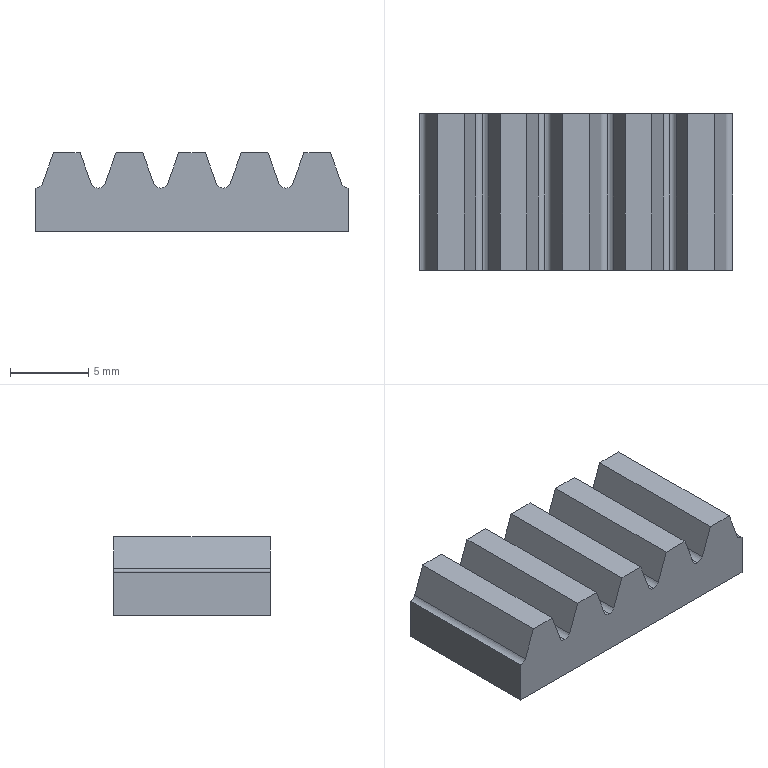Part | SolidWorks | features Cut 1, MBimport 1 | 1 solid | 33 faces | box 20 x 10 x 5 mm | volume 819.626 mm3 | plane 21 | cylinder 12 | commonest cylinder face diameters 0.959 x10 3.18 x2
STEP:
#1=CARTESIAN_POINT('',(13.656,4.812,2.));
#2=VERTEX_POINT('',#1);
#3=CARTESIAN_POINT('',(10.476,4.812,2.));
#4=VERTEX_POINT('',#3);
#5=CARTESIAN_POINT('',(12.066,4.812,2.));
#6=DIRECTION('',(0.,0.,-1.));
#7=DIRECTION('',(-1.,0.,0.));
#8=AXIS2_PLACEMENT_3D('',#5,#6,#7);
#9=CIRCLE('',#8,1.59);
#10=EDGE_CURVE('',#2,#4,#9,.T.);
#11=ORIENTED_EDGE('',*,*,#10,.F.);
#12=CARTESIAN_POINT('',(13.656,4.812,0.));
#13=VERTEX_POINT('',#12);
#14=CARTESIAN_POINT('',(13.656,4.812,2.));
#15=DIRECTION('',(0.,0.,-1.));
#16=VECTOR('',#15,1000.);
#17=LINE('',#14,#16);
#18=EDGE_CURVE('',#2,#13,#17,.T.);
#19=ORIENTED_EDGE('',*,*,#18,.T.);
#20=CARTESIAN_POINT('',(10.476,4.812,0.));
#21=VERTEX_POINT('',#20);
#22=CARTESIAN_POINT('',(12.066,4.812,0.));
#23=DIRECTION('',(0.,0.,-1.));
#24=DIRECTION('',(-1.,0.,0.));
#25=AXIS2_PLACEMENT_3D('',#22,#23,#24);
#26=CIRCLE('',#25,1.59);
#27=EDGE_CURVE('',#13,#21,#26,.T.);
#28=ORIENTED_EDGE('',*,*,#27,.T.);
#29=CARTESIAN_POINT('',(10.476,4.812,2.));
#30=DIRECTION('',(0.,0.,-1.));
#31=VECTOR('',#30,1000.);
#32=LINE('',#29,#31);
#33=EDGE_CURVE('',#4,#21,#32,.T.);
#34=ORIENTED_EDGE('',*,*,#33,.F.);
#35=EDGE_LOOP('',(#11,#19,#28,#34));
#36=FACE_OUTER_BOUND('',#35,.T.);
#37=CARTESIAN_POINT('',(12.066,4.812,2.));
#38=DIRECTION('',(0.,0.,-1.));
#39=DIRECTION('',(-1.,0.,0.));
#40=AXIS2_PLACEMENT_3D('',#37,#38,#39);
#41=CYLINDRICAL_SURFACE('',#40,1.59);
#42=ADVANCED_FACE('',(#36),#41,.F.);
#43=CARTESIAN_POINT('',(4.,10.,2.75));
#44=VERTEX_POINT('',#43);
#45=CARTESIAN_POINT('',(4.421,10.,3.));
#46=VERTEX_POINT('',#45);
#47=CARTESIAN_POINT('',(4.,10.,3.23));
#48=DIRECTION('',(0.,-1.,0.));
#49=DIRECTION('',(0.,0.,1.));
#50=AXIS2_PLACEMENT_3D('',#47,#48,#49);
#51=CIRCLE('',#50,0.4795);
#52=EDGE_CURVE('',#44,#46,#51,.T.);
#53=ORIENTED_EDGE('',*,*,#52,.F.);
#54=CARTESIAN_POINT('',(4.,0.,2.75));
#55=VERTEX_POINT('',#54);
#56=CARTESIAN_POINT('',(4.,22.913,2.75));
#57=DIRECTION('',(0.,-1.,0.));
#58=VECTOR('',#57,1000.);
#59=LINE('',#56,#58);
#60=EDGE_CURVE('',#44,#55,#59,.T.);
#61=ORIENTED_EDGE('',*,*,#60,.T.);
#62=CARTESIAN_POINT('',(4.421,0.,3.));
#63=VERTEX_POINT('',#62);
#64=CARTESIAN_POINT('',(4.,0.,3.23));
#65=DIRECTION('',(0.,1.,0.));
#66=DIRECTION('',(1.,0.,0.));
#67=AXIS2_PLACEMENT_3D('',#64,#65,#66);
#68=CIRCLE('',#67,0.4795);
#69=EDGE_CURVE('',#63,#55,#68,.T.);
#70=ORIENTED_EDGE('',*,*,#69,.F.);
#71=CARTESIAN_POINT('',(4.421,22.913,3.));
#72=DIRECTION('',(0.,-1.,0.));
#73=VECTOR('',#72,1000.);
#74=LINE('',#71,#73);
#75=EDGE_CURVE('',#46,#63,#74,.T.);
#76=ORIENTED_EDGE('',*,*,#75,.F.);
#77=EDGE_LOOP('',(#53,#61,#70,#76));
#78=FACE_OUTER_BOUND('',#77,.T.);
#79=CARTESIAN_POINT('',(4.,22.913,3.23));
#80=DIRECTION('',(0.,-1.,0.));
#81=DIRECTION('',(0.,0.,-1.));
#82=AXIS2_PLACEMENT_3D('',#79,#80,#81);
#83=CYLINDRICAL_SURFACE('',#82,0.4795);
#84=ADVANCED_FACE('',(#78),#83,.F.);
#85=CARTESIAN_POINT('',(8.,10.,2.75));
#86=VERTEX_POINT('',#85);
#87=CARTESIAN_POINT('',(8.421,10.,3.));
#88=VERTEX_POINT('',#87);
#89=CARTESIAN_POINT('',(8.,10.,3.23));
#90=DIRECTION('',(0.,-1.,0.));
#91=DIRECTION('',(0.,0.,1.));
#92=AXIS2_PLACEMENT_3D('',#89,#90,#91);
#93=CIRCLE('',#92,0.4795);
#94=EDGE_CURVE('',#86,#88,#93,.T.);
#95=ORIENTED_EDGE('',*,*,#94,.F.);
#96=CARTESIAN_POINT('',(8.,0.,2.75));
#97=VERTEX_POINT('',#96);
#98=CARTESIAN_POINT('',(8.,22.913,2.75));
#99=DIRECTION('',(0.,-1.,0.));
#100=VECTOR('',#99,1000.);
#101=LINE('',#98,#100);
#102=EDGE_CURVE('',#86,#97,#101,.T.);
#103=ORIENTED_EDGE('',*,*,#102,.T.);
#104=CARTESIAN_POINT('',(8.421,0.,3.));
#105=VERTEX_POINT('',#104);
#106=CARTESIAN_POINT('',(8.,0.,3.23));
#107=DIRECTION('',(0.,1.,0.));
#108=DIRECTION('',(1.,0.,0.));
#109=AXIS2_PLACEMENT_3D('',#106,#107,#108);
#110=CIRCLE('',#109,0.4795);
#111=EDGE_CURVE('',#105,#97,#110,.T.);
#112=ORIENTED_EDGE('',*,*,#111,.F.);
#113=CARTESIAN_POINT('',(8.421,22.913,3.));
#114=DIRECTION('',(0.,-1.,0.));
#115=VECTOR('',#114,1000.);
#116=LINE('',#113,#115);
#117=EDGE_CURVE('',#88,#105,#116,.T.);
#118=ORIENTED_EDGE('',*,*,#117,.F.);
#119=EDGE_LOOP('',(#95,#103,#112,#118));
#120=FACE_OUTER_BOUND('',#119,.T.);
#121=CARTESIAN_POINT('',(8.,22.913,3.23));
#122=DIRECTION('',(0.,-1.,0.));
#123=DIRECTION('',(0.,0.,-1.));
#124=AXIS2_PLACEMENT_3D('',#121,#122,#123);
#125=CYLINDRICAL_SURFACE('',#124,0.4795);
#126=ADVANCED_FACE('',(#120),#125,.F.);
#127=CARTESIAN_POINT('',(12.,10.,2.75));
#128=VERTEX_POINT('',#127);
#129=CARTESIAN_POINT('',(12.421,10.,3.));
#130=VERTEX_POINT('',#129);
#131=CARTESIAN_POINT('',(12.,10.,3.23));
#132=DIRECTION('',(0.,-1.,0.));
#133=DIRECTION('',(0.,0.,1.));
#134=AXIS2_PLACEMENT_3D('',#131,#132,#133);
#135=CIRCLE('',#134,0.4795);
#136=EDGE_CURVE('',#128,#130,#135,.T.);
#137=ORIENTED_EDGE('',*,*,#136,.F.);
#138=CARTESIAN_POINT('',(12.,0.,2.75));
#139=VERTEX_POINT('',#138);
#140=CARTESIAN_POINT('',(12.,22.913,2.75));
#141=DIRECTION('',(0.,-1.,0.));
#142=VECTOR('',#141,1000.);
#143=LINE('',#140,#142);
#144=EDGE_CURVE('',#128,#139,#143,.T.);
#145=ORIENTED_EDGE('',*,*,#144,.T.);
#146=CARTESIAN_POINT('',(12.421,0.,3.));
#147=VERTEX_POINT('',#146);
#148=CARTESIAN_POINT('',(12.,0.,3.23));
#149=DIRECTION('',(0.,1.,0.));
#150=DIRECTION('',(1.,0.,0.));
#151=AXIS2_PLACEMENT_3D('',#148,#149,#150);
#152=CIRCLE('',#151,0.4795);
#153=EDGE_CURVE('',#147,#139,#152,.T.);
#154=ORIENTED_EDGE('',*,*,#153,.F.);
#155=CARTESIAN_POINT('',(12.421,22.913,3.));
#156=DIRECTION('',(0.,-1.,0.));
#157=VECTOR('',#156,1000.);
#158=LINE('',#155,#157);
#159=EDGE_CURVE('',#130,#147,#158,.T.);
#160=ORIENTED_EDGE('',*,*,#159,.F.);
#161=EDGE_LOOP('',(#137,#145,#154,#160));
#162=FACE_OUTER_BOUND('',#161,.T.);
#163=CARTESIAN_POINT('',(12.,22.913,3.23));
#164=DIRECTION('',(0.,-1.,0.));
#165=DIRECTION('',(0.,0.,-1.));
#166=AXIS2_PLACEMENT_3D('',#163,#164,#165);
#167=CYLINDRICAL_SURFACE('',#166,0.4795);
#168=ADVANCED_FACE('',(#162),#167,.F.);
#169=CARTESIAN_POINT('',(16.,10.,2.75));
#170=VERTEX_POINT('',#169);
#171=CARTESIAN_POINT('',(16.421,10.,3.));
#172=VERTEX_POINT('',#171);
#173=CARTESIAN_POINT('',(16.,10.,3.23));
#174=DIRECTION('',(0.,-1.,0.));
#175=DIRECTION('',(0.,0.,1.));
#176=AXIS2_PLACEMENT_3D('',#173,#174,#175);
#177=CIRCLE('',#176,0.4795);
#178=EDGE_CURVE('',#170,#172,#177,.T.);
#179=ORIENTED_EDGE('',*,*,#178,.F.);
#180=CARTESIAN_POINT('',(16.,0.,2.75));
#181=VERTEX_POINT('',#180);
#182=CARTESIAN_POINT('',(16.,22.913,2.75));
#183=DIRECTION('',(0.,-1.,0.));
#184=VECTOR('',#183,1000.);
#185=LINE('',#182,#184);
#186=EDGE_CURVE('',#170,#181,#185,.T.);
#187=ORIENTED_EDGE('',*,*,#186,.T.);
#188=CARTESIAN_POINT('',(16.421,0.,3.));
#189=VERTEX_POINT('',#188);
#190=CARTESIAN_POINT('',(16.,0.,3.23));
#191=DIRECTION('',(0.,1.,0.));
#192=DIRECTION('',(1.,0.,0.));
#193=AXIS2_PLACEMENT_3D('',#190,#191,#192);
#194=CIRCLE('',#193,0.4795);
#195=EDGE_CURVE('',#189,#181,#194,.T.);
#196=ORIENTED_EDGE('',*,*,#195,.F.);
#197=CARTESIAN_POINT('',(16.421,22.913,3.));
#198=DIRECTION('',(0.,-1.,0.));
#199=VECTOR('',#198,1000.);
#200=LINE('',#197,#199);
#201=EDGE_CURVE('',#172,#189,#200,.T.);
#202=ORIENTED_EDGE('',*,*,#201,.F.);
#203=EDGE_LOOP('',(#179,#187,#196,#202));
#204=FACE_OUTER_BOUND('',#203,.T.);
#205=CARTESIAN_POINT('',(16.,22.913,3.23));
#206=DIRECTION('',(0.,-1.,0.));
#207=DIRECTION('',(0.,0.,-1.));
#208=AXIS2_PLACEMENT_3D('',#205,#206,#207);
#209=CYLINDRICAL_SURFACE('',#208,0.4795);
#210=ADVANCED_FACE('',(#204),#209,.F.);
#211=CARTESIAN_POINT('',(20.,0.,2.75));
#212=VERTEX_POINT('',#211);
#213=CARTESIAN_POINT('',(20.,10.,2.75));
#214=VERTEX_POINT('',#213);
#215=CARTESIAN_POINT('',(20.,23.922,2.75));
#216=DIRECTION('',(0.,1.,0.));
#217=VECTOR('',#216,1000.);
#218=LINE('',#215,#217);
#219=EDGE_CURVE('',#212,#214,#218,.T.);
#220=ORIENTED_EDGE('',*,*,#219,.T.);
#221=CARTESIAN_POINT('',(19.579,10.,3.));
#222=VERTEX_POINT('',#221);
#223=CARTESIAN_POINT('',(20.,10.,3.23));
#224=DIRECTION('',(0.,-1.,0.));
#225=DIRECTION('',(0.,0.,1.));
#226=AXIS2_PLACEMENT_3D('',#223,#224,#225);
#227=CIRCLE('',#226,0.4795);
#228=EDGE_CURVE('',#222,#214,#227,.T.);
#229=ORIENTED_EDGE('',*,*,#228,.F.);
#230=CARTESIAN_POINT('',(19.579,0.,3.));
#231=VERTEX_POINT('',#230);
#232=CARTESIAN_POINT('',(19.579,23.922,3.));
#233=DIRECTION('',(0.,-1.,0.));
#234=VECTOR('',#233,1000.);
#235=LINE('',#232,#234);
#236=EDGE_CURVE('',#222,#231,#235,.T.);
#237=ORIENTED_EDGE('',*,*,#236,.T.);
#238=CARTESIAN_POINT('',(20.,0.,3.23));
#239=DIRECTION('',(0.,-1.,0.));
#240=DIRECTION('',(0.,0.,1.));
#241=AXIS2_PLACEMENT_3D('',#238,#239,#240);
#242=CIRCLE('',#241,0.4795);
#243=EDGE_CURVE('',#231,#212,#242,.T.);
#244=ORIENTED_EDGE('',*,*,#243,.T.);
#245=EDGE_LOOP('',(#220,#229,#237,#244));
#246=FACE_OUTER_BOUND('',#245,.T.);
#247=CARTESIAN_POINT('',(20.,23.922,3.23));
#248=DIRECTION('',(0.,-1.,0.));
#249=DIRECTION('',(0.,0.,-1.));
#250=AXIS2_PLACEMENT_3D('',#247,#248,#249);
#251=CYLINDRICAL_SURFACE('',#250,0.4795);
#252=ADVANCED_FACE('',(#246),#251,.F.);
#253=CARTESIAN_POINT('',(18.851,10.,5.));
#254=VERTEX_POINT('',#253);
#255=CARTESIAN_POINT('',(18.851,0.,5.));
#256=VERTEX_POINT('',#255);
#257=CARTESIAN_POINT('',(18.851,23.922,5.));
#258=DIRECTION('',(0.,-1.,0.));
#259=VECTOR('',#258,1000.);
#260=LINE('',#257,#259);
#261=EDGE_CURVE('',#254,#256,#260,.T.);
#262=ORIENTED_EDGE('',*,*,#261,.T.);
#263=CARTESIAN_POINT('',(19.579,0.,3.));
#264=DIRECTION('',(-0.342,0.,0.9397));
#265=VECTOR('',#264,1000.);
#266=LINE('',#263,#265);
#267=EDGE_CURVE('',#231,#256,#266,.T.);
#268=ORIENTED_EDGE('',*,*,#267,.F.);
#269=ORIENTED_EDGE('',*,*,#236,.F.);
#270=CARTESIAN_POINT('',(18.253,10.,6.643));
#271=DIRECTION('',(0.342,0.,-0.9397));
#272=VECTOR('',#271,1000.);
#273=LINE('',#270,#272);
#274=EDGE_CURVE('',#254,#222,#273,.T.);
#275=ORIENTED_EDGE('',*,*,#274,.F.);
#276=EDGE_LOOP('',(#262,#268,#269,#275));
#277=FACE_OUTER_BOUND('',#276,.T.);
#278=CARTESIAN_POINT('',(19.579,23.922,3.));
#279=DIRECTION('',(0.9397,0.,0.342));
#280=DIRECTION('',(0.,-1.,0.));
#281=AXIS2_PLACEMENT_3D('',#278,#279,#280);
#282=PLANE('',#281);
#283=ADVANCED_FACE('',(#277),#282,.T.);
#284=ORIENTED_EDGE('',*,*,#186,.F.);
#285=CARTESIAN_POINT('',(15.579,10.,3.));
#286=VERTEX_POINT('',#285);
#287=CARTESIAN_POINT('',(16.,10.,3.23));
#288=DIRECTION('',(0.,-1.,0.));
#289=DIRECTION('',(0.,0.,1.));
#290=AXIS2_PLACEMENT_3D('',#287,#288,#289);
#291=CIRCLE('',#290,0.4795);
#292=EDGE_CURVE('',#286,#170,#291,.T.);
#293=ORIENTED_EDGE('',*,*,#292,.F.);
#294=CARTESIAN_POINT('',(15.579,0.,3.));
#295=VERTEX_POINT('',#294);
#296=CARTESIAN_POINT('',(15.579,22.913,3.));
#297=DIRECTION('',(0.,-1.,0.));
#298=VECTOR('',#297,1000.);
#299=LINE('',#296,#298);
#300=EDGE_CURVE('',#286,#295,#299,.T.);
#301=ORIENTED_EDGE('',*,*,#300,.T.);
#302=CARTESIAN_POINT('',(16.,0.,3.23));
#303=DIRECTION('',(0.,1.,0.));
#304=DIRECTION('',(1.,0.,0.));
#305=AXIS2_PLACEMENT_3D('',#302,#303,#304);
#306=CIRCLE('',#305,0.4795);
#307=EDGE_CURVE('',#181,#295,#306,.T.);
#308=ORIENTED_EDGE('',*,*,#307,.F.);
#309=EDGE_LOOP('',(#284,#293,#301,#308));
#310=FACE_OUTER_BOUND('',#309,.T.);
#311=CARTESIAN_POINT('',(16.,22.913,3.23));
#312=DIRECTION('',(0.,-1.,0.));
#313=DIRECTION('',(0.,0.,-1.));
#314=AXIS2_PLACEMENT_3D('',#311,#312,#313);
#315=CYLINDRICAL_SURFACE('',#314,0.4795);
#316=ADVANCED_FACE('',(#310),#315,.F.);
#317=ORIENTED_EDGE('',*,*,#201,.T.);
#318=CARTESIAN_POINT('',(17.149,0.,5.));
#319=VERTEX_POINT('',#318);
#320=CARTESIAN_POINT('',(16.421,0.,3.));
#321=DIRECTION('',(-0.342,0.,-0.9397));
#322=VECTOR('',#321,1000.);
#323=LINE('',#320,#322);
#324=EDGE_CURVE('',#319,#189,#323,.T.);
#325=ORIENTED_EDGE('',*,*,#324,.F.);
#326=CARTESIAN_POINT('',(17.149,10.,5.));
#327=VERTEX_POINT('',#326);
#328=CARTESIAN_POINT('',(17.149,22.913,5.));
#329=DIRECTION('',(0.,-1.,0.));
#330=VECTOR('',#329,1000.);
#331=LINE('',#328,#330);
#332=EDGE_CURVE('',#327,#319,#331,.T.);
#333=ORIENTED_EDGE('',*,*,#332,.F.);
#334=CARTESIAN_POINT('',(13.536,10.,-4.927));
#335=DIRECTION('',(0.342,0.,0.9397));
#336=VECTOR('',#335,1000.);
#337=LINE('',#334,#336);
#338=EDGE_CURVE('',#172,#327,#337,.T.);
#339=ORIENTED_EDGE('',*,*,#338,.F.);
#340=EDGE_LOOP('',(#317,#325,#333,#339));
#341=FACE_OUTER_BOUND('',#340,.T.);
#342=CARTESIAN_POINT('',(16.421,22.913,3.));
#343=DIRECTION('',(-0.9397,0.,0.342));
#344=DIRECTION('',(0.,1.,0.));
#345=AXIS2_PLACEMENT_3D('',#342,#343,#344);
#346=PLANE('',#345);
#347=ADVANCED_FACE('',(#341),#346,.T.);
#348=CARTESIAN_POINT('',(14.851,10.,5.));
#349=VERTEX_POINT('',#348);
#350=CARTESIAN_POINT('',(14.851,0.,5.));
#351=VERTEX_POINT('',#350);
#352=CARTESIAN_POINT('',(14.851,22.913,5.));
#353=DIRECTION('',(0.,-1.,0.));
#354=VECTOR('',#353,1000.);
#355=LINE('',#352,#354);
#356=EDGE_CURVE('',#349,#351,#355,.T.);
#357=ORIENTED_EDGE('',*,*,#356,.T.);
#358=CARTESIAN_POINT('',(15.579,0.,3.));
#359=DIRECTION('',(-0.342,0.,0.9397));
#360=VECTOR('',#359,1000.);
#361=LINE('',#358,#360);
#362=EDGE_CURVE('',#295,#351,#361,.T.);
#363=ORIENTED_EDGE('',*,*,#362,.F.);
#364=ORIENTED_EDGE('',*,*,#300,.F.);
#365=CARTESIAN_POINT('',(14.721,10.,5.358));
#366=DIRECTION('',(0.342,0.,-0.9397));
#367=VECTOR('',#366,1000.);
#368=LINE('',#365,#367);
#369=EDGE_CURVE('',#349,#286,#368,.T.);
#370=ORIENTED_EDGE('',*,*,#369,.F.);
#371=EDGE_LOOP('',(#357,#363,#364,#370));
#372=FACE_OUTER_BOUND('',#371,.T.);
#373=CARTESIAN_POINT('',(15.579,22.913,3.));
#374=DIRECTION('',(0.9397,0.,0.342));
#375=DIRECTION('',(0.,-1.,0.));
#376=AXIS2_PLACEMENT_3D('',#373,#374,#375);
#377=PLANE('',#376);
#378=ADVANCED_FACE('',(#372),#377,.T.);
#379=ORIENTED_EDGE('',*,*,#144,.F.);
#380=CARTESIAN_POINT('',(11.579,10.,3.));
#381=VERTEX_POINT('',#380);
#382=CARTESIAN_POINT('',(12.,10.,3.23));
#383=DIRECTION('',(0.,-1.,0.));
#384=DIRECTION('',(0.,0.,1.));
#385=AXIS2_PLACEMENT_3D('',#382,#383,#384);
#386=CIRCLE('',#385,0.4795);
#387=EDGE_CURVE('',#381,#128,#386,.T.);
#388=ORIENTED_EDGE('',*,*,#387,.F.);
#389=CARTESIAN_POINT('',(11.579,0.,3.));
#390=VERTEX_POINT('',#389);
#391=CARTESIAN_POINT('',(11.579,22.913,3.));
#392=DIRECTION('',(0.,-1.,0.));
#393=VECTOR('',#392,1000.);
#394=LINE('',#391,#393);
#395=EDGE_CURVE('',#381,#390,#394,.T.);
#396=ORIENTED_EDGE('',*,*,#395,.T.);
#397=CARTESIAN_POINT('',(12.,0.,3.23));
#398=DIRECTION('',(0.,1.,0.));
#399=DIRECTION('',(1.,0.,0.));
#400=AXIS2_PLACEMENT_3D('',#397,#398,#399);
#401=CIRCLE('',#400,0.4795);
#402=EDGE_CURVE('',#139,#390,#401,.T.);
#403=ORIENTED_EDGE('',*,*,#402,.F.);
#404=EDGE_LOOP('',(#379,#388,#396,#403));
#405=FACE_OUTER_BOUND('',#404,.T.);
#406=CARTESIAN_POINT('',(12.,22.913,3.23));
#407=DIRECTION('',(0.,-1.,0.));
#408=DIRECTION('',(0.,0.,-1.));
#409=AXIS2_PLACEMENT_3D('',#406,#407,#408);
#410=CYLINDRICAL_SURFACE('',#409,0.4795);
#411=ADVANCED_FACE('',(#405),#410,.F.);
#412=ORIENTED_EDGE('',*,*,#159,.T.);
#413=CARTESIAN_POINT('',(13.149,0.,5.));
#414=VERTEX_POINT('',#413);
#415=CARTESIAN_POINT('',(12.421,0.,3.));
#416=DIRECTION('',(-0.342,0.,-0.9397));
#417=VECTOR('',#416,1000.);
#418=LINE('',#415,#417);
#419=EDGE_CURVE('',#414,#147,#418,.T.);
#420=ORIENTED_EDGE('',*,*,#419,.F.);
#421=CARTESIAN_POINT('',(13.149,10.,5.));
#422=VERTEX_POINT('',#421);
#423=CARTESIAN_POINT('',(13.149,22.913,5.));
#424=DIRECTION('',(0.,-1.,0.));
#425=VECTOR('',#424,1000.);
#426=LINE('',#423,#425);
#427=EDGE_CURVE('',#422,#414,#426,.T.);
#428=ORIENTED_EDGE('',*,*,#427,.F.);
#429=CARTESIAN_POINT('',(10.004,10.,-3.641));
#430=DIRECTION('',(0.342,0.,0.9397));
#431=VECTOR('',#430,1000.);
#432=LINE('',#429,#431);
#433=EDGE_CURVE('',#130,#422,#432,.T.);
#434=ORIENTED_EDGE('',*,*,#433,.F.);
#435=EDGE_LOOP('',(#412,#420,#428,#434));
#436=FACE_OUTER_BOUND('',#435,.T.);
#437=CARTESIAN_POINT('',(12.421,22.913,3.));
#438=DIRECTION('',(-0.9397,0.,0.342));
#439=DIRECTION('',(0.,1.,0.));
#440=AXIS2_PLACEMENT_3D('',#437,#438,#439);
#441=PLANE('',#440);
#442=ADVANCED_FACE('',(#436),#441,.T.);
#443=CARTESIAN_POINT('',(10.851,10.,5.));
#444=VERTEX_POINT('',#443);
#445=CARTESIAN_POINT('',(10.851,0.,5.));
#446=VERTEX_POINT('',#445);
#447=CARTESIAN_POINT('',(10.851,22.913,5.));
#448=DIRECTION('',(0.,-1.,0.));
#449=VECTOR('',#448,1000.);
#450=LINE('',#447,#449);
#451=EDGE_CURVE('',#444,#446,#450,.T.);
#452=ORIENTED_EDGE('',*,*,#451,.T.);
#453=CARTESIAN_POINT('',(11.579,0.,3.));
#454=DIRECTION('',(-0.342,0.,0.9397));
#455=VECTOR('',#454,1000.);
#456=LINE('',#453,#455);
#457=EDGE_CURVE('',#390,#446,#456,.T.);
#458=ORIENTED_EDGE('',*,*,#457,.F.);
#459=ORIENTED_EDGE('',*,*,#395,.F.);
#460=CARTESIAN_POINT('',(11.189,10.,4.072));
#461=DIRECTION('',(0.342,0.,-0.9397));
#462=VECTOR('',#461,1000.);
#463=LINE('',#460,#462);
#464=EDGE_CURVE('',#444,#381,#463,.T.);
#465=ORIENTED_EDGE('',*,*,#464,.F.);
#466=EDGE_LOOP('',(#452,#458,#459,#465));
#467=FACE_OUTER_BOUND('',#466,.T.);
#468=CARTESIAN_POINT('',(11.579,22.913,3.));
#469=DIRECTION('',(0.9397,0.,0.342));
#470=DIRECTION('',(0.,-1.,0.));
#471=AXIS2_PLACEMENT_3D('',#468,#469,#470);
#472=PLANE('',#471);
#473=ADVANCED_FACE('',(#467),#472,.T.);
#474=ORIENTED_EDGE('',*,*,#102,.F.);
#475=CARTESIAN_POINT('',(7.579,10.,3.));
#476=VERTEX_POINT('',#475);
#477=CARTESIAN_POINT('',(8.,10.,3.23));
#478=DIRECTION('',(0.,-1.,0.));
#479=DIRECTION('',(0.,0.,1.));
#480=AXIS2_PLACEMENT_3D('',#477,#478,#479);
#481=CIRCLE('',#480,0.4795);
#482=EDGE_CURVE('',#476,#86,#481,.T.);
#483=ORIENTED_EDGE('',*,*,#482,.F.);
#484=CARTESIAN_POINT('',(7.579,0.,3.));
#485=VERTEX_POINT('',#484);
#486=CARTESIAN_POINT('',(7.579,22.913,3.));
#487=DIRECTION('',(0.,-1.,0.));
#488=VECTOR('',#487,1000.);
#489=LINE('',#486,#488);
#490=EDGE_CURVE('',#476,#485,#489,.T.);
#491=ORIENTED_EDGE('',*,*,#490,.T.);
#492=CARTESIAN_POINT('',(8.,0.,3.23));
#493=DIRECTION('',(0.,1.,0.));
#494=DIRECTION('',(1.,0.,0.));
#495=AXIS2_PLACEMENT_3D('',#492,#493,#494);
#496=CIRCLE('',#495,0.4795);
#497=EDGE_CURVE('',#97,#485,#496,.T.);
#498=ORIENTED_EDGE('',*,*,#497,.F.);
#499=EDGE_LOOP('',(#474,#483,#491,#498));
#500=FACE_OUTER_BOUND('',#499,.T.);
#501=CARTESIAN_POINT('',(8.,22.913,3.23));
#502=DIRECTION('',(0.,-1.,0.));
#503=DIRECTION('',(0.,0.,-1.));
#504=AXIS2_PLACEMENT_3D('',#501,#502,#503);
#505=CYLINDRICAL_SURFACE('',#504,0.4795);
#506=ADVANCED_FACE('',(#500),#505,.F.);
#507=ORIENTED_EDGE('',*,*,#117,.T.);
#508=CARTESIAN_POINT('',(9.149,0.,5.));
#509=VERTEX_POINT('',#508);
#510=CARTESIAN_POINT('',(8.421,0.,3.));
#511=DIRECTION('',(-0.342,0.,-0.9397));
#512=VECTOR('',#511,1000.);
#513=LINE('',#510,#512);
#514=EDGE_CURVE('',#509,#105,#513,.T.);
#515=ORIENTED_EDGE('',*,*,#514,.F.);
#516=CARTESIAN_POINT('',(9.149,10.,5.));
#517=VERTEX_POINT('',#516);
#518=CARTESIAN_POINT('',(9.149,22.913,5.));
#519=DIRECTION('',(0.,-1.,0.));
#520=VECTOR('',#519,1000.);
#521=LINE('',#518,#520);
#522=EDGE_CURVE('',#517,#509,#521,.T.);
#523=ORIENTED_EDGE('',*,*,#522,.F.);
#524=CARTESIAN_POINT('',(6.472,10.,-2.356));
#525=DIRECTION('',(0.342,0.,0.9397));
#526=VECTOR('',#525,1000.);
#527=LINE('',#524,#526);
#528=EDGE_CURVE('',#88,#517,#527,.T.);
#529=ORIENTED_EDGE('',*,*,#528,.F.);
#530=EDGE_LOOP('',(#507,#515,#523,#529));
#531=FACE_OUTER_BOUND('',#530,.T.);
#532=CARTESIAN_POINT('',(8.421,22.913,3.));
#533=DIRECTION('',(-0.9397,0.,0.342));
#534=DIRECTION('',(0.,1.,0.));
#535=AXIS2_PLACEMENT_3D('',#532,#533,#534);
#536=PLANE('',#535);
#537=ADVANCED_FACE('',(#531),#536,.T.);
#538=CARTESIAN_POINT('',(6.851,10.,5.));
#539=VERTEX_POINT('',#538);
#540=CARTESIAN_POINT('',(6.851,0.,5.));
#541=VERTEX_POINT('',#540);
#542=CARTESIAN_POINT('',(6.851,22.913,5.));
#543=DIRECTION('',(0.,-1.,0.));
#544=VECTOR('',#543,1000.);
#545=LINE('',#542,#544);
#546=EDGE_CURVE('',#539,#541,#545,.T.);
#547=ORIENTED_EDGE('',*,*,#546,.T.);
#548=CARTESIAN_POINT('',(7.579,0.,3.));
#549=DIRECTION('',(-0.342,0.,0.9397));
#550=VECTOR('',#549,1000.);
#551=LINE('',#548,#550);
#552=EDGE_CURVE('',#485,#541,#551,.T.);
#553=ORIENTED_EDGE('',*,*,#552,.F.);
#554=ORIENTED_EDGE('',*,*,#490,.F.);
#555=CARTESIAN_POINT('',(7.657,10.,2.787));
#556=DIRECTION('',(0.342,0.,-0.9397));
#557=VECTOR('',#556,1000.);
#558=LINE('',#555,#557);
#559=EDGE_CURVE('',#539,#476,#558,.T.);
#560=ORIENTED_EDGE('',*,*,#559,.F.);
#561=EDGE_LOOP('',(#547,#553,#554,#560));
#562=FACE_OUTER_BOUND('',#561,.T.);
#563=CARTESIAN_POINT('',(7.579,22.913,3.));
#564=DIRECTION('',(0.9397,0.,0.342));
#565=DIRECTION('',(0.,-1.,0.));
#566=AXIS2_PLACEMENT_3D('',#563,#564,#565);
#567=PLANE('',#566);
#568=ADVANCED_FACE('',(#562),#567,.T.);
#569=ORIENTED_EDGE('',*,*,#60,.F.);
#570=CARTESIAN_POINT('',(3.579,10.,3.));
#571=VERTEX_POINT('',#570);
#572=CARTESIAN_POINT('',(4.,10.,3.23));
#573=DIRECTION('',(0.,-1.,0.));
#574=DIRECTION('',(0.,0.,1.));
#575=AXIS2_PLACEMENT_3D('',#572,#573,#574);
#576=CIRCLE('',#575,0.4795);
#577=EDGE_CURVE('',#571,#44,#576,.T.);
#578=ORIENTED_EDGE('',*,*,#577,.F.);
#579=CARTESIAN_POINT('',(3.579,0.,3.));
#580=VERTEX_POINT('',#579);
#581=CARTESIAN_POINT('',(3.579,22.913,3.));
#582=DIRECTION('',(0.,-1.,0.));
#583=VECTOR('',#582,1000.);
#584=LINE('',#581,#583);
#585=EDGE_CURVE('',#571,#580,#584,.T.);
#586=ORIENTED_EDGE('',*,*,#585,.T.);
#587=CARTESIAN_POINT('',(4.,0.,3.23));
#588=DIRECTION('',(0.,1.,0.));
#589=DIRECTION('',(1.,0.,0.));
#590=AXIS2_PLACEMENT_3D('',#587,#588,#589);
#591=CIRCLE('',#590,0.4795);
#592=EDGE_CURVE('',#55,#580,#591,.T.);
#593=ORIENTED_EDGE('',*,*,#592,.F.);
#594=EDGE_LOOP('',(#569,#578,#586,#593));
#595=FACE_OUTER_BOUND('',#594,.T.);
#596=CARTESIAN_POINT('',(4.,22.913,3.23));
#597=DIRECTION('',(0.,-1.,0.));
#598=DIRECTION('',(0.,0.,-1.));
#599=AXIS2_PLACEMENT_3D('',#596,#597,#598);
#600=CYLINDRICAL_SURFACE('',#599,0.4795);
#601=ADVANCED_FACE('',(#595),#600,.F.);
#602=ORIENTED_EDGE('',*,*,#75,.T.);
#603=CARTESIAN_POINT('',(5.149,0.,5.));
#604=VERTEX_POINT('',#603);
#605=CARTESIAN_POINT('',(4.421,0.,3.));
#606=DIRECTION('',(-0.342,0.,-0.9397));
#607=VECTOR('',#606,1000.);
#608=LINE('',#605,#607);
#609=EDGE_CURVE('',#604,#63,#608,.T.);
#610=ORIENTED_EDGE('',*,*,#609,.F.);
#611=CARTESIAN_POINT('',(5.149,10.,5.));
#612=VERTEX_POINT('',#611);
#613=CARTESIAN_POINT('',(5.149,22.913,5.));
#614=DIRECTION('',(0.,-1.,0.));
#615=VECTOR('',#614,1000.);
#616=LINE('',#613,#615);
#617=EDGE_CURVE('',#612,#604,#616,.T.);
#618=ORIENTED_EDGE('',*,*,#617,.F.);
#619=CARTESIAN_POINT('',(2.94,10.,-1.07));
#620=DIRECTION('',(0.342,0.,0.9397));
#621=VECTOR('',#620,1000.);
#622=LINE('',#619,#621);
#623=EDGE_CURVE('',#46,#612,#622,.T.);
#624=ORIENTED_EDGE('',*,*,#623,.F.);
#625=EDGE_LOOP('',(#602,#610,#618,#624));
#626=FACE_OUTER_BOUND('',#625,.T.);
#627=CARTESIAN_POINT('',(4.421,22.913,3.));
#628=DIRECTION('',(-0.9397,0.,0.342));
#629=DIRECTION('',(0.,1.,0.));
#630=AXIS2_PLACEMENT_3D('',#627,#628,#629);
#631=PLANE('',#630);
#632=ADVANCED_FACE('',(#626),#631,.T.);
#633=CARTESIAN_POINT('',(2.851,10.,5.));
#634=VERTEX_POINT('',#633);
#635=CARTESIAN_POINT('',(2.851,0.,5.));
#636=VERTEX_POINT('',#635);
#637=CARTESIAN_POINT('',(2.851,22.913,5.));
#638=DIRECTION('',(0.,-1.,0.));
#639=VECTOR('',#638,1000.);
#640=LINE('',#637,#639);
#641=EDGE_CURVE('',#634,#636,#640,.T.);
#642=ORIENTED_EDGE('',*,*,#641,.T.);
#643=CARTESIAN_POINT('',(3.579,0.,3.));
#644=DIRECTION('',(-0.342,0.,0.9397));
#645=VECTOR('',#644,1000.);
#646=LINE('',#643,#645);
#647=EDGE_CURVE('',#580,#636,#646,.T.);
#648=ORIENTED_EDGE('',*,*,#647,.F.);
#649=ORIENTED_EDGE('',*,*,#585,.F.);
#650=CARTESIAN_POINT('',(4.124,10.,1.501));
#651=DIRECTION('',(0.342,0.,-0.9397));
#652=VECTOR('',#651,1000.);
#653=LINE('',#650,#652);
#654=EDGE_CURVE('',#634,#571,#653,.T.);
#655=ORIENTED_EDGE('',*,*,#654,.F.);
#656=EDGE_LOOP('',(#642,#648,#649,#655));
#657=FACE_OUTER_BOUND('',#656,.T.);
#658=CARTESIAN_POINT('',(3.579,22.913,3.));
#659=DIRECTION('',(0.9397,0.,0.342));
#660=DIRECTION('',(0.,-1.,0.));
#661=AXIS2_PLACEMENT_3D('',#658,#659,#660);
#662=PLANE('',#661);
#663=ADVANCED_FACE('',(#657),#662,.T.);
#664=CARTESIAN_POINT('',(0.,10.,2.75));
#665=VERTEX_POINT('',#664);
#666=CARTESIAN_POINT('',(0.,0.,2.75));
#667=VERTEX_POINT('',#666);
#668=CARTESIAN_POINT('',(0.,23.922,2.75));
#669=DIRECTION('',(0.,-1.,0.));
#670=VECTOR('',#669,1000.);
#671=LINE('',#668,#670);
#672=EDGE_CURVE('',#665,#667,#671,.T.);
#673=ORIENTED_EDGE('',*,*,#672,.T.);
#674=CARTESIAN_POINT('',(0.421,0.,3.));
#675=VERTEX_POINT('',#674);
#676=CARTESIAN_POINT('',(0.,0.,3.23));
#677=DIRECTION('',(0.,1.,0.));
#678=DIRECTION('',(1.,0.,0.));
#679=AXIS2_PLACEMENT_3D('',#676,#677,#678);
#680=CIRCLE('',#679,0.4795);
#681=EDGE_CURVE('',#675,#667,#680,.T.);
#682=ORIENTED_EDGE('',*,*,#681,.F.);
#683=CARTESIAN_POINT('',(0.421,10.,3.));
#684=VERTEX_POINT('',#683);
#685=CARTESIAN_POINT('',(0.421,23.922,3.));
#686=DIRECTION('',(0.,-1.,0.));
#687=VECTOR('',#686,1000.);
#688=LINE('',#685,#687);
#689=EDGE_CURVE('',#684,#675,#688,.T.);
#690=ORIENTED_EDGE('',*,*,#689,.F.);
#691=CARTESIAN_POINT('',(0.,10.,3.23));
#692=DIRECTION('',(0.,-1.,0.));
#693=DIRECTION('',(0.,0.,1.));
#694=AXIS2_PLACEMENT_3D('',#691,#692,#693);
#695=CIRCLE('',#694,0.4795);
#696=EDGE_CURVE('',#665,#684,#695,.T.);
#697=ORIENTED_EDGE('',*,*,#696,.F.);
#698=EDGE_LOOP('',(#673,#682,#690,#697));
#699=FACE_OUTER_BOUND('',#698,.T.);
#700=CARTESIAN_POINT('',(0.,23.922,3.23));
#701=DIRECTION('',(0.,-1.,0.));
#702=DIRECTION('',(0.,0.,-1.));
#703=AXIS2_PLACEMENT_3D('',#700,#701,#702);
#704=CYLINDRICAL_SURFACE('',#703,0.4795);
#705=ADVANCED_FACE('',(#699),#704,.F.);
#706=ORIENTED_EDGE('',*,*,#689,.T.);
#707=CARTESIAN_POINT('',(1.149,0.,5.));
#708=VERTEX_POINT('',#707);
#709=CARTESIAN_POINT('',(0.421,0.,3.));
#710=DIRECTION('',(-0.342,0.,-0.9397));
#711=VECTOR('',#710,1000.);
#712=LINE('',#709,#711);
#713=EDGE_CURVE('',#708,#675,#712,.T.);
#714=ORIENTED_EDGE('',*,*,#713,.F.);
#715=CARTESIAN_POINT('',(1.149,10.,5.));
#716=VERTEX_POINT('',#715);
#717=CARTESIAN_POINT('',(1.149,23.922,5.));
#718=DIRECTION('',(0.,-1.,0.));
#719=VECTOR('',#718,1000.);
#720=LINE('',#717,#719);
#721=EDGE_CURVE('',#716,#708,#720,.T.);
#722=ORIENTED_EDGE('',*,*,#721,.F.);
#723=CARTESIAN_POINT('',(-0.5924,10.,0.2156));
#724=DIRECTION('',(0.342,0.,0.9397));
#725=VECTOR('',#724,1000.);
#726=LINE('',#723,#725);
#727=EDGE_CURVE('',#684,#716,#726,.T.);
#728=ORIENTED_EDGE('',*,*,#727,.F.);
#729=EDGE_LOOP('',(#706,#714,#722,#728));
#730=FACE_OUTER_BOUND('',#729,.T.);
#731=CARTESIAN_POINT('',(0.421,23.922,3.));
#732=DIRECTION('',(-0.9397,0.,0.342));
#733=DIRECTION('',(0.,1.,0.));
#734=AXIS2_PLACEMENT_3D('',#731,#732,#733);
#735=PLANE('',#734);
#736=ADVANCED_FACE('',(#730),#735,.T.);
#737=ORIENTED_EDGE('',*,*,#267,.T.);
#738=CARTESIAN_POINT('',(0.,0.,5.));
#739=DIRECTION('',(1.,0.,0.));
#740=VECTOR('',#739,1000.);
#741=LINE('',#738,#740);
#742=EDGE_CURVE('',#319,#256,#741,.T.);
#743=ORIENTED_EDGE('',*,*,#742,.F.);
#744=ORIENTED_EDGE('',*,*,#324,.T.);
#745=ORIENTED_EDGE('',*,*,#195,.T.);
#746=ORIENTED_EDGE('',*,*,#307,.T.);
#747=ORIENTED_EDGE('',*,*,#362,.T.);
#748=CARTESIAN_POINT('',(0.,0.,5.));
#749=DIRECTION('',(1.,0.,0.));
#750=VECTOR('',#749,1000.);
#751=LINE('',#748,#750);
#752=EDGE_CURVE('',#414,#351,#751,.T.);
#753=ORIENTED_EDGE('',*,*,#752,.F.);
#754=ORIENTED_EDGE('',*,*,#419,.T.);
#755=ORIENTED_EDGE('',*,*,#153,.T.);
#756=ORIENTED_EDGE('',*,*,#402,.T.);
#757=ORIENTED_EDGE('',*,*,#457,.T.);
#758=CARTESIAN_POINT('',(0.,0.,5.));
#759=DIRECTION('',(1.,0.,0.));
#760=VECTOR('',#759,1000.);
#761=LINE('',#758,#760);
#762=EDGE_CURVE('',#509,#446,#761,.T.);
#763=ORIENTED_EDGE('',*,*,#762,.F.);
#764=ORIENTED_EDGE('',*,*,#514,.T.);
#765=ORIENTED_EDGE('',*,*,#111,.T.);
#766=ORIENTED_EDGE('',*,*,#497,.T.);
#767=ORIENTED_EDGE('',*,*,#552,.T.);
#768=CARTESIAN_POINT('',(0.,0.,5.));
#769=DIRECTION('',(1.,0.,0.));
#770=VECTOR('',#769,1000.);
#771=LINE('',#768,#770);
#772=EDGE_CURVE('',#604,#541,#771,.T.);
#773=ORIENTED_EDGE('',*,*,#772,.F.);
#774=ORIENTED_EDGE('',*,*,#609,.T.);
#775=ORIENTED_EDGE('',*,*,#69,.T.);
#776=ORIENTED_EDGE('',*,*,#592,.T.);
#777=ORIENTED_EDGE('',*,*,#647,.T.);
#778=CARTESIAN_POINT('',(0.,0.,5.));
#779=DIRECTION('',(1.,0.,0.));
#780=VECTOR('',#779,1000.);
#781=LINE('',#778,#780);
#782=EDGE_CURVE('',#708,#636,#781,.T.);
#783=ORIENTED_EDGE('',*,*,#782,.F.);
#784=ORIENTED_EDGE('',*,*,#713,.T.);
#785=ORIENTED_EDGE('',*,*,#681,.T.);
#786=CARTESIAN_POINT('',(0.,0.,0.));
#787=VERTEX_POINT('',#786);
#788=CARTESIAN_POINT('',(0.,0.,5.));
#789=DIRECTION('',(0.,0.,1.));
#790=VECTOR('',#789,1000.);
#791=LINE('',#788,#790);
#792=EDGE_CURVE('',#787,#667,#791,.T.);
#793=ORIENTED_EDGE('',*,*,#792,.F.);
#794=CARTESIAN_POINT('',(20.,0.,0.));
#795=VERTEX_POINT('',#794);
#796=CARTESIAN_POINT('',(0.,0.,0.));
#797=DIRECTION('',(-1.,0.,0.));
#798=VECTOR('',#797,1000.);
#799=LINE('',#796,#798);
#800=EDGE_CURVE('',#795,#787,#799,.T.);
#801=ORIENTED_EDGE('',*,*,#800,.F.);
#802=CARTESIAN_POINT('',(20.,0.,5.));
#803=DIRECTION('',(0.,0.,-1.));
#804=VECTOR('',#803,1000.);
#805=LINE('',#802,#804);
#806=EDGE_CURVE('',#212,#795,#805,.T.);
#807=ORIENTED_EDGE('',*,*,#806,.F.);
#808=ORIENTED_EDGE('',*,*,#243,.F.);
#809=EDGE_LOOP('',(#737,#743,#744,#745,#746,#747,#753,#754,#755,#756,#757,#763,#764,#765,#766,#767,#773,#774,#775,#776,#777,#783,#784,#785,#793,#801,#807,#808));
#810=FACE_OUTER_BOUND('',#809,.T.);
#811=CARTESIAN_POINT('',(0.,0.,0.));
#812=DIRECTION('',(0.,1.,0.));
#813=DIRECTION('',(1.,0.,0.));
#814=AXIS2_PLACEMENT_3D('',#811,#812,#813);
#815=PLANE('',#814);
#816=ADVANCED_FACE('',(#810),#815,.F.);
#817=CARTESIAN_POINT('',(0.,10.,5.));
#818=DIRECTION('',(1.,0.,0.));
#819=VECTOR('',#818,1000.);
#820=LINE('',#817,#819);
#821=EDGE_CURVE('',#327,#254,#820,.T.);
#822=ORIENTED_EDGE('',*,*,#821,.T.);
#823=ORIENTED_EDGE('',*,*,#274,.T.);
#824=ORIENTED_EDGE('',*,*,#228,.T.);
#825=CARTESIAN_POINT('',(20.,10.,0.));
#826=VERTEX_POINT('',#825);
#827=CARTESIAN_POINT('',(20.,10.,5.));
#828=DIRECTION('',(0.,0.,-1.));
#829=VECTOR('',#828,1000.);
#830=LINE('',#827,#829);
#831=EDGE_CURVE('',#214,#826,#830,.T.);
#832=ORIENTED_EDGE('',*,*,#831,.T.);
#833=CARTESIAN_POINT('',(0.,10.,0.));
#834=VERTEX_POINT('',#833);
#835=CARTESIAN_POINT('',(0.,10.,0.));
#836=DIRECTION('',(-1.,0.,0.));
#837=VECTOR('',#836,1000.);
#838=LINE('',#835,#837);
#839=EDGE_CURVE('',#826,#834,#838,.T.);
#840=ORIENTED_EDGE('',*,*,#839,.T.);
#841=CARTESIAN_POINT('',(0.,10.,5.));
#842=DIRECTION('',(0.,0.,1.));
#843=VECTOR('',#842,1000.);
#844=LINE('',#841,#843);
#845=EDGE_CURVE('',#834,#665,#844,.T.);
#846=ORIENTED_EDGE('',*,*,#845,.T.);
#847=ORIENTED_EDGE('',*,*,#696,.T.);
#848=ORIENTED_EDGE('',*,*,#727,.T.);
#849=CARTESIAN_POINT('',(0.,10.,5.));
#850=DIRECTION('',(1.,0.,0.));
#851=VECTOR('',#850,1000.);
#852=LINE('',#849,#851);
#853=EDGE_CURVE('',#716,#634,#852,.T.);
#854=ORIENTED_EDGE('',*,*,#853,.T.);
#855=ORIENTED_EDGE('',*,*,#654,.T.);
#856=ORIENTED_EDGE('',*,*,#577,.T.);
#857=ORIENTED_EDGE('',*,*,#52,.T.);
#858=ORIENTED_EDGE('',*,*,#623,.T.);
#859=CARTESIAN_POINT('',(0.,10.,5.));
#860=DIRECTION('',(1.,0.,0.));
#861=VECTOR('',#860,1000.);
#862=LINE('',#859,#861);
#863=EDGE_CURVE('',#612,#539,#862,.T.);
#864=ORIENTED_EDGE('',*,*,#863,.T.);
#865=ORIENTED_EDGE('',*,*,#559,.T.);
#866=ORIENTED_EDGE('',*,*,#482,.T.);
#867=ORIENTED_EDGE('',*,*,#94,.T.);
#868=ORIENTED_EDGE('',*,*,#528,.T.);
#869=CARTESIAN_POINT('',(0.,10.,5.));
#870=DIRECTION('',(1.,0.,0.));
#871=VECTOR('',#870,1000.);
#872=LINE('',#869,#871);
#873=EDGE_CURVE('',#517,#444,#872,.T.);
#874=ORIENTED_EDGE('',*,*,#873,.T.);
#875=ORIENTED_EDGE('',*,*,#464,.T.);
#876=ORIENTED_EDGE('',*,*,#387,.T.);
#877=ORIENTED_EDGE('',*,*,#136,.T.);
#878=ORIENTED_EDGE('',*,*,#433,.T.);
#879=CARTESIAN_POINT('',(0.,10.,5.));
#880=DIRECTION('',(1.,0.,0.));
#881=VECTOR('',#880,1000.);
#882=LINE('',#879,#881);
#883=EDGE_CURVE('',#422,#349,#882,.T.);
#884=ORIENTED_EDGE('',*,*,#883,.T.);
#885=ORIENTED_EDGE('',*,*,#369,.T.);
#886=ORIENTED_EDGE('',*,*,#292,.T.);
#887=ORIENTED_EDGE('',*,*,#178,.T.);
#888=ORIENTED_EDGE('',*,*,#338,.T.);
#889=EDGE_LOOP('',(#822,#823,#824,#832,#840,#846,#847,#848,#854,#855,#856,#857,#858,#864,#865,#866,#867,#868,#874,#875,#876,#877,#878,#884,#885,#886,#887,#888));
#890=FACE_OUTER_BOUND('',#889,.T.);
#891=CARTESIAN_POINT('',(0.,10.,0.));
#892=DIRECTION('',(0.,1.,0.));
#893=DIRECTION('',(1.,0.,0.));
#894=AXIS2_PLACEMENT_3D('',#891,#892,#893);
#895=PLANE('',#894);
#896=ADVANCED_FACE('',(#890),#895,.T.);
#897=CARTESIAN_POINT('',(12.066,4.812,0.));
#898=DIRECTION('',(0.,0.,-1.));
#899=DIRECTION('',(-1.,0.,0.));
#900=AXIS2_PLACEMENT_3D('',#897,#898,#899);
#901=CIRCLE('',#900,1.59);
#902=EDGE_CURVE('',#21,#13,#901,.T.);
#903=ORIENTED_EDGE('',*,*,#902,.F.);
#904=ORIENTED_EDGE('',*,*,#27,.F.);
#905=EDGE_LOOP('',(#903,#904));
#906=FACE_BOUND('',#905,.T.);
#907=ORIENTED_EDGE('',*,*,#800,.T.);
#908=CARTESIAN_POINT('',(0.,10.,0.));
#909=DIRECTION('',(0.,-1.,0.));
#910=VECTOR('',#909,1000.);
#911=LINE('',#908,#910);
#912=EDGE_CURVE('',#834,#787,#911,.T.);
#913=ORIENTED_EDGE('',*,*,#912,.F.);
#914=ORIENTED_EDGE('',*,*,#839,.F.);
#915=CARTESIAN_POINT('',(20.,10.,0.));
#916=DIRECTION('',(0.,-1.,0.));
#917=VECTOR('',#916,1000.);
#918=LINE('',#915,#917);
#919=EDGE_CURVE('',#826,#795,#918,.T.);
#920=ORIENTED_EDGE('',*,*,#919,.T.);
#921=EDGE_LOOP('',(#907,#913,#914,#920));
#922=FACE_OUTER_BOUND('',#921,.T.);
#923=CARTESIAN_POINT('',(0.,10.,0.));
#924=DIRECTION('',(0.,0.,1.));
#925=DIRECTION('',(1.,0.,0.));
#926=AXIS2_PLACEMENT_3D('',#923,#924,#925);
#927=PLANE('',#926);
#928=ADVANCED_FACE('',(#906,#922),#927,.F.);
#929=ORIENTED_EDGE('',*,*,#672,.F.);
#930=ORIENTED_EDGE('',*,*,#845,.F.);
#931=ORIENTED_EDGE('',*,*,#912,.T.);
#932=ORIENTED_EDGE('',*,*,#792,.T.);
#933=EDGE_LOOP('',(#929,#930,#931,#932));
#934=FACE_OUTER_BOUND('',#933,.T.);
#935=CARTESIAN_POINT('',(0.,10.,5.));
#936=DIRECTION('',(1.,0.,0.));
#937=DIRECTION('',(0.,1.,0.));
#938=AXIS2_PLACEMENT_3D('',#935,#936,#937);
#939=PLANE('',#938);
#940=ADVANCED_FACE('',(#934),#939,.F.);
#941=ORIENTED_EDGE('',*,*,#641,.F.);
#942=ORIENTED_EDGE('',*,*,#853,.F.);
#943=ORIENTED_EDGE('',*,*,#721,.T.);
#944=ORIENTED_EDGE('',*,*,#782,.T.);
#945=EDGE_LOOP('',(#941,#942,#943,#944));
#946=FACE_OUTER_BOUND('',#945,.T.);
#947=CARTESIAN_POINT('',(0.,10.,5.));
#948=DIRECTION('',(0.,0.,-1.));
#949=DIRECTION('',(0.,-1.,0.));
#950=AXIS2_PLACEMENT_3D('',#947,#948,#949);
#951=PLANE('',#950);
#952=ADVANCED_FACE('',(#946),#951,.F.);
#953=ORIENTED_EDGE('',*,*,#546,.F.);
#954=ORIENTED_EDGE('',*,*,#863,.F.);
#955=ORIENTED_EDGE('',*,*,#617,.T.);
#956=ORIENTED_EDGE('',*,*,#772,.T.);
#957=EDGE_LOOP('',(#953,#954,#955,#956));
#958=FACE_OUTER_BOUND('',#957,.T.);
#959=CARTESIAN_POINT('',(0.,10.,5.));
#960=DIRECTION('',(0.,0.,-1.));
#961=DIRECTION('',(0.,-1.,0.));
#962=AXIS2_PLACEMENT_3D('',#959,#960,#961);
#963=PLANE('',#962);
#964=ADVANCED_FACE('',(#958),#963,.F.);
#965=ORIENTED_EDGE('',*,*,#451,.F.);
#966=ORIENTED_EDGE('',*,*,#873,.F.);
#967=ORIENTED_EDGE('',*,*,#522,.T.);
#968=ORIENTED_EDGE('',*,*,#762,.T.);
#969=EDGE_LOOP('',(#965,#966,#967,#968));
#970=FACE_OUTER_BOUND('',#969,.T.);
#971=CARTESIAN_POINT('',(0.,10.,5.));
#972=DIRECTION('',(0.,0.,-1.));
#973=DIRECTION('',(0.,-1.,0.));
#974=AXIS2_PLACEMENT_3D('',#971,#972,#973);
#975=PLANE('',#974);
#976=ADVANCED_FACE('',(#970),#975,.F.);
#977=ORIENTED_EDGE('',*,*,#356,.F.);
#978=ORIENTED_EDGE('',*,*,#883,.F.);
#979=ORIENTED_EDGE('',*,*,#427,.T.);
#980=ORIENTED_EDGE('',*,*,#752,.T.);
#981=EDGE_LOOP('',(#977,#978,#979,#980));
#982=FACE_OUTER_BOUND('',#981,.T.);
#983=CARTESIAN_POINT('',(0.,10.,5.));
#984=DIRECTION('',(0.,0.,-1.));
#985=DIRECTION('',(0.,-1.,0.));
#986=AXIS2_PLACEMENT_3D('',#983,#984,#985);
#987=PLANE('',#986);
#988=ADVANCED_FACE('',(#982),#987,.F.);
#989=ORIENTED_EDGE('',*,*,#219,.F.);
#990=ORIENTED_EDGE('',*,*,#806,.T.);
#991=ORIENTED_EDGE('',*,*,#919,.F.);
#992=ORIENTED_EDGE('',*,*,#831,.F.);
#993=EDGE_LOOP('',(#989,#990,#991,#992));
#994=FACE_OUTER_BOUND('',#993,.T.);
#995=CARTESIAN_POINT('',(20.,10.,5.));
#996=DIRECTION('',(-1.,0.,0.));
#997=DIRECTION('',(0.,0.,1.));
#998=AXIS2_PLACEMENT_3D('',#995,#996,#997);
#999=PLANE('',#998);
#1000=ADVANCED_FACE('',(#994),#999,.F.);
#1001=ORIENTED_EDGE('',*,*,#261,.F.);
#1002=ORIENTED_EDGE('',*,*,#821,.F.);
#1003=ORIENTED_EDGE('',*,*,#332,.T.);
#1004=ORIENTED_EDGE('',*,*,#742,.T.);
#1005=EDGE_LOOP('',(#1001,#1002,#1003,#1004));
#1006=FACE_OUTER_BOUND('',#1005,.T.);
#1007=CARTESIAN_POINT('',(0.,10.,5.));
#1008=DIRECTION('',(0.,0.,-1.));
#1009=DIRECTION('',(0.,-1.,0.));
#1010=AXIS2_PLACEMENT_3D('',#1007,#1008,#1009);
#1011=PLANE('',#1010);
#1012=ADVANCED_FACE('',(#1006),#1011,.F.);
#1013=ORIENTED_EDGE('',*,*,#18,.F.);
#1014=CARTESIAN_POINT('',(12.066,4.812,2.));
#1015=DIRECTION('',(0.,0.,-1.));
#1016=DIRECTION('',(-1.,0.,0.));
#1017=AXIS2_PLACEMENT_3D('',#1014,#1015,#1016);
#1018=CIRCLE('',#1017,1.59);
#1019=EDGE_CURVE('',#4,#2,#1018,.T.);
#1020=ORIENTED_EDGE('',*,*,#1019,.F.);
#1021=ORIENTED_EDGE('',*,*,#33,.T.);
#1022=ORIENTED_EDGE('',*,*,#902,.T.);
#1023=EDGE_LOOP('',(#1013,#1020,#1021,#1022));
#1024=FACE_OUTER_BOUND('',#1023,.T.);
#1025=CARTESIAN_POINT('',(12.066,4.812,2.));
#1026=DIRECTION('',(0.,0.,-1.));
#1027=DIRECTION('',(-1.,0.,0.));
#1028=AXIS2_PLACEMENT_3D('',#1025,#1026,#1027);
#1029=CYLINDRICAL_SURFACE('',#1028,1.59);
#1030=ADVANCED_FACE('',(#1024),#1029,.F.);
#1031=ORIENTED_EDGE('',*,*,#1019,.T.);
#1032=ORIENTED_EDGE('',*,*,#10,.T.);
#1033=EDGE_LOOP('',(#1031,#1032));
#1034=FACE_OUTER_BOUND('',#1033,.T.);
#1035=CARTESIAN_POINT('',(12.066,4.812,2.));
#1036=DIRECTION('',(0.,0.,-1.));
#1037=DIRECTION('',(-1.,0.,0.));
#1038=AXIS2_PLACEMENT_3D('',#1035,#1036,#1037);
#1039=PLANE('',#1038);
#1040=ADVANCED_FACE('',(#1034),#1039,.T.);
#1041=CLOSED_SHELL('',(#42,#84,#126,#168,#210,#252,#283,#316,#347,#378,#411,#442,#473,#506,#537,#568,#601,#632,#663,#705,#736,#816,#896,#928,#940,#952,#964,#976,#988,#1000,#1012,#1030,#1040));
#1042=MANIFOLD_SOLID_BREP('',#1041);
#1043=CARTESIAN_POINT('',(0.,0.,0.));
#1044=DIRECTION('',(0.,0.,1.));
#1045=DIRECTION('',(1.,0.,0.));
#1046=AXIS2_PLACEMENT_3D('',#1043,#1044,#1045);
#1047=(LENGTH_UNIT()NAMED_UNIT(*)SI_UNIT(.MILLI.,.METRE.));
#1048=UNCERTAINTY_MEASURE_WITH_UNIT(LENGTH_MEASURE(0.00001),#1047,'','');
#1049=(NAMED_UNIT(*)PLANE_ANGLE_UNIT()SI_UNIT($,.RADIAN.));
#1050=(NAMED_UNIT(*)SI_UNIT($,.STERADIAN.)SOLID_ANGLE_UNIT());
#1051=(GEOMETRIC_REPRESENTATION_CONTEXT(3)GLOBAL_UNCERTAINTY_ASSIGNED_CONTEXT((#1048))GLOBAL_UNIT_ASSIGNED_CONTEXT((#1047,#1049,#1050))REPRESENTATION_CONTEXT('',''));
#1052=ADVANCED_BREP_SHAPE_REPRESENTATION('',(#1042,#1046),#1051);